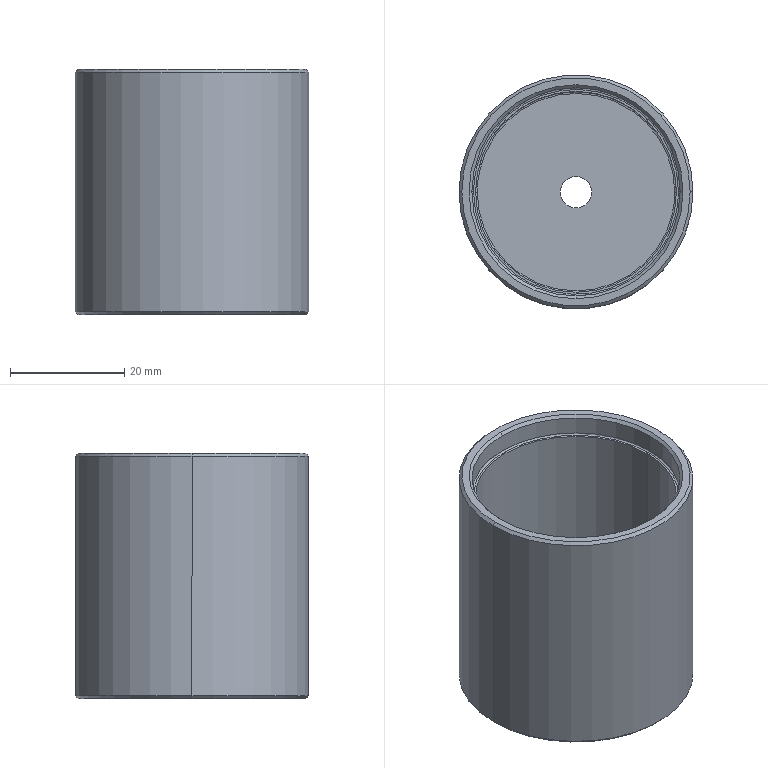Part | STEP file | Inner collar ring | 1 solid | 24 faces | box 41 x 41 x 43 mm | volume 18386 mm3 | cylinder 8 | cone 8 | spline 4 | plane 4 | commonest cylinder face diameters 5.5 x2 35.2 x2 36.5 x2 41 x2